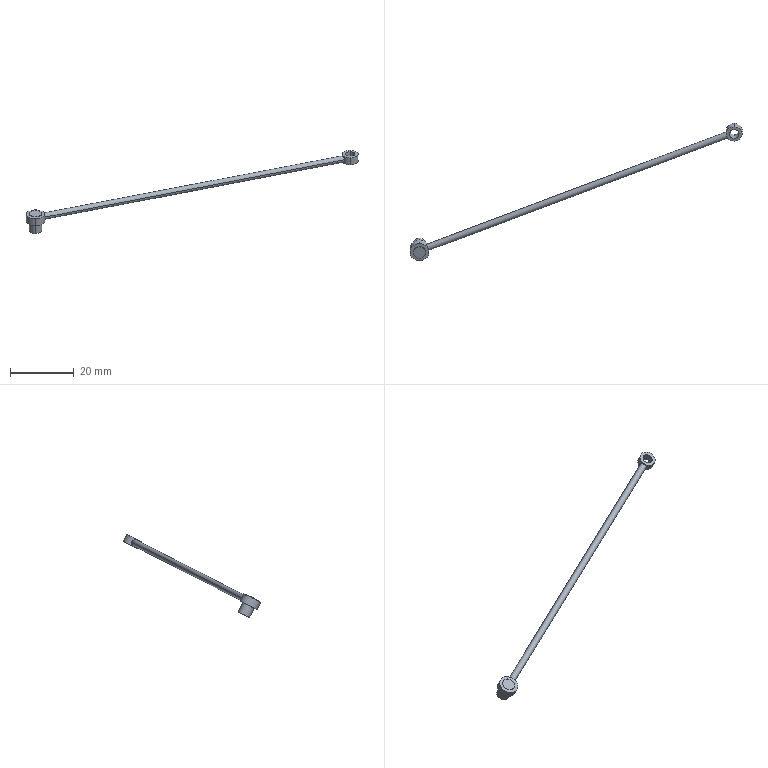Part | STEP file | Completa.sldasm-Part-147_Valor predeterminado | 1 solid | 18 faces | box 104.527 x 43.22 x 26.157 mm | volume 466.69 mm3 | cylinder 12 | plane 6 | commonest cylinder face diameters 4 x4 2 x2 3 x2 5 x2 6 x2